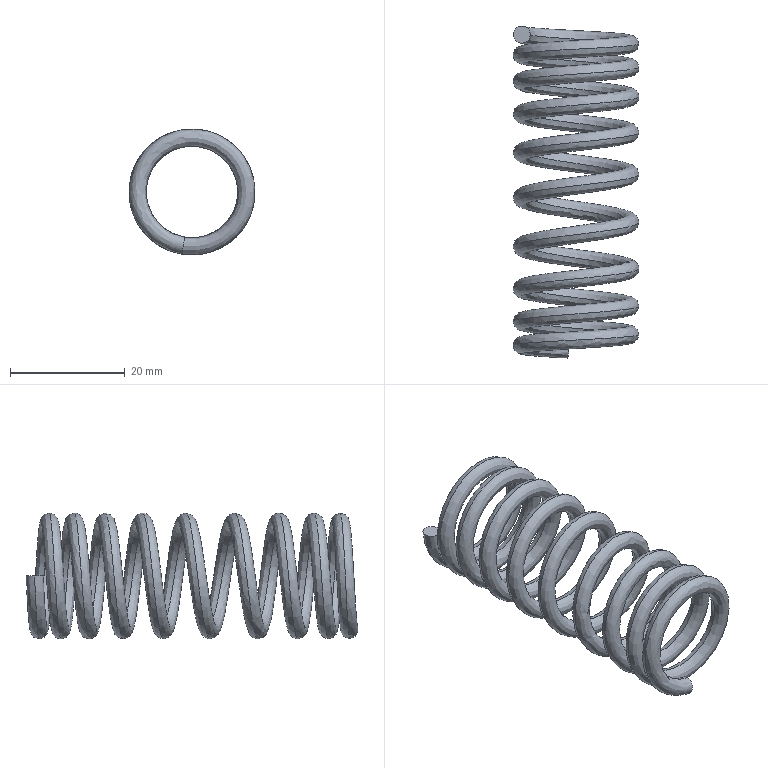Part | SolidWorks | features Helix 1, Sweep 1 | 1 solid | 4 faces | box 22 x 58 x 22 mm | volume 3891 mm3 | spline 2 | plane 2